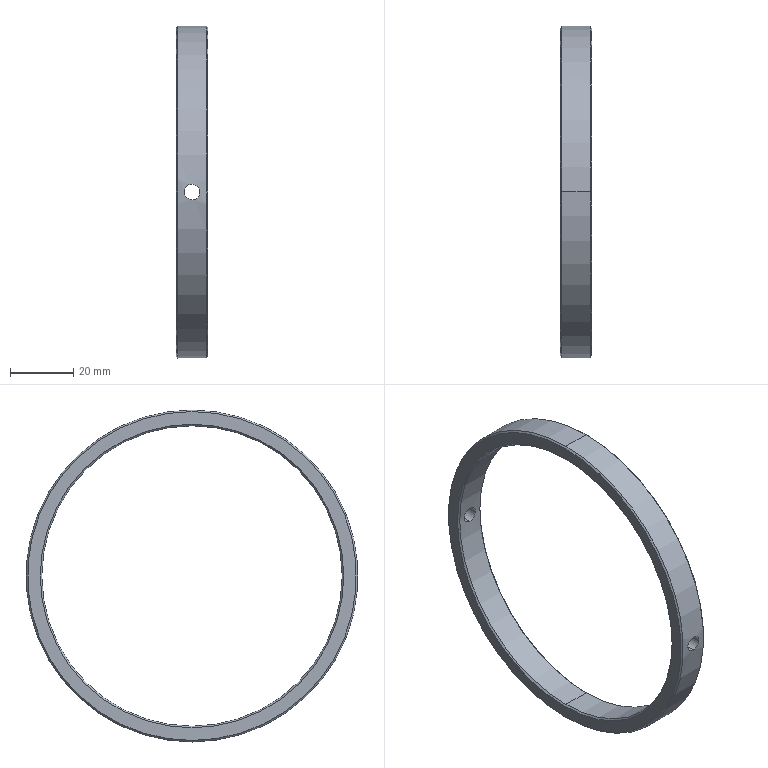Part | SolidWorks | features Chamfer 1, Extrusion 1, HoleWzd 1 | 1 solid | 18 faces | box 10 x 105 x 105 mm | volume 15354 mm3 | cylinder 8 | cone 8 | plane 2 | commonest cylinder face diameters 5 x4 95 x2 105 x2
STEP:
#1=CARTESIAN_POINT('',(0.,-52.44,-2.5));
#2=VERTEX_POINT('',#1);
#3=CARTESIAN_POINT('',(0.,-52.44,2.5));
#4=VERTEX_POINT('',#3);
#5=CARTESIAN_POINT('',(0.,-52.44,-2.5));
#6=CARTESIAN_POINT('',(-0.1649,-52.44,-2.5));
#7=CARTESIAN_POINT('',(-0.3279,-52.441,-2.484));
#8=CARTESIAN_POINT('',(-0.6473,-52.444,-2.42));
#9=CARTESIAN_POINT('',(-0.8058,-52.446,-2.372));
#10=CARTESIAN_POINT('',(-1.109,-52.452,-2.247));
#11=CARTESIAN_POINT('',(-1.252,-52.455,-2.17));
#12=CARTESIAN_POINT('',(-1.524,-52.462,-1.989));
#13=CARTESIAN_POINT('',(-1.653,-52.466,-1.883));
#14=CARTESIAN_POINT('',(-1.883,-52.474,-1.652));
#15=CARTESIAN_POINT('',(-1.987,-52.478,-1.526));
#16=CARTESIAN_POINT('',(-2.169,-52.485,-1.254));
#17=CARTESIAN_POINT('',(-2.247,-52.489,-1.108));
#18=CARTESIAN_POINT('',(-2.434,-52.497,-0.6566));
#19=CARTESIAN_POINT('',(-2.5,-52.5,-0.3283));
#20=CARTESIAN_POINT('',(-2.5,-52.5,0.1671));
#21=CARTESIAN_POINT('',(-2.484,-52.499,0.3295));
#22=CARTESIAN_POINT('',(-2.42,-52.496,0.6489));
#23=CARTESIAN_POINT('',(-2.372,-52.494,0.8076));
#24=CARTESIAN_POINT('',(-2.246,-52.488,1.11));
#25=CARTESIAN_POINT('',(-2.169,-52.485,1.254));
#26=CARTESIAN_POINT('',(-1.987,-52.478,1.525));
#27=CARTESIAN_POINT('',(-1.882,-52.474,1.654));
#28=CARTESIAN_POINT('',(-1.651,-52.466,1.884));
#29=CARTESIAN_POINT('',(-1.525,-52.462,1.988));
#30=CARTESIAN_POINT('',(-1.252,-52.455,2.17));
#31=CARTESIAN_POINT('',(-1.106,-52.452,2.248));
#32=CARTESIAN_POINT('',(-0.8055,-52.446,2.372));
#33=CARTESIAN_POINT('',(-0.6479,-52.444,2.42));
#34=CARTESIAN_POINT('',(-0.3252,-52.441,2.484));
#35=CARTESIAN_POINT('',(-0.163,-52.44,2.5));
#36=CARTESIAN_POINT('',(0.,-52.44,2.5));
#37=B_SPLINE_CURVE_WITH_KNOTS('',3,(#5,#6,#7,#8,#9,#10,#11,#12,#13,#14,#15,#16,#17,#18,#19,#20,#21,#22,#23,#24,#25,#26,#27,#28,#29,#30,#31,#32,#33,#34,#35,#36),.UNSPECIFIED.,.F.,.F.,(4,2,2,2,2,2,2,2,2,2,2,2,2,2,2,4),(0.01173,0.01222,0.0127,0.01319,0.01368,0.01417,0.01466,0.01563,0.01612,0.01661,0.0171,0.01759,0.01808,0.01857,0.01905,0.01954),.UNSPECIFIED.);
#38=EDGE_CURVE('',#2,#4,#37,.T.);
#39=ORIENTED_EDGE('',*,*,#38,.F.);
#40=CARTESIAN_POINT('',(0.,-47.434,-2.5));
#41=VERTEX_POINT('',#40);
#42=CARTESIAN_POINT('',(0.,52.5,-2.5));
#43=DIRECTION('',(0.,1.,0.));
#44=VECTOR('',#43,1000.);
#45=LINE('',#42,#44);
#46=EDGE_CURVE('',#2,#41,#45,.T.);
#47=ORIENTED_EDGE('',*,*,#46,.T.);
#48=CARTESIAN_POINT('',(0.,-47.434,2.5));
#49=VERTEX_POINT('',#48);
#50=CARTESIAN_POINT('',(0.,-47.434,-2.5));
#51=CARTESIAN_POINT('',(-0.1631,-47.434,-2.5));
#52=CARTESIAN_POINT('',(-0.3253,-47.435,-2.484));
#53=CARTESIAN_POINT('',(-0.6476,-47.438,-2.42));
#54=CARTESIAN_POINT('',(-0.8056,-47.441,-2.372));
#55=CARTESIAN_POINT('',(-1.257,-47.45,-2.185));
#56=CARTESIAN_POINT('',(-1.536,-47.458,-1.999));
#57=CARTESIAN_POINT('',(-1.882,-47.471,-1.654));
#58=CARTESIAN_POINT('',(-1.987,-47.476,-1.525));
#59=CARTESIAN_POINT('',(-2.169,-47.484,-1.254));
#60=CARTESIAN_POINT('',(-2.246,-47.487,-1.11));
#61=CARTESIAN_POINT('',(-2.372,-47.493,-0.8078));
#62=CARTESIAN_POINT('',(-2.42,-47.496,-0.6488));
#63=CARTESIAN_POINT('',(-2.484,-47.499,-0.3293));
#64=CARTESIAN_POINT('',(-2.5,-47.5,-0.167));
#65=CARTESIAN_POINT('',(-2.5,-47.5,0.1629));
#66=CARTESIAN_POINT('',(-2.484,-47.499,0.3259));
#67=CARTESIAN_POINT('',(-2.421,-47.496,0.6454));
#68=CARTESIAN_POINT('',(-2.373,-47.493,0.8039));
#69=CARTESIAN_POINT('',(-2.248,-47.487,1.107));
#70=CARTESIAN_POINT('',(-2.171,-47.484,1.251));
#71=CARTESIAN_POINT('',(-1.99,-47.476,1.522));
#72=CARTESIAN_POINT('',(-1.884,-47.471,1.651));
#73=CARTESIAN_POINT('',(-1.654,-47.463,1.882));
#74=CARTESIAN_POINT('',(-1.528,-47.459,1.985));
#75=CARTESIAN_POINT('',(-1.255,-47.451,2.168));
#76=CARTESIAN_POINT('',(-1.11,-47.447,2.246));
#77=CARTESIAN_POINT('',(-0.6585,-47.438,2.434));
#78=CARTESIAN_POINT('',(-0.3303,-47.434,2.5));
#79=CARTESIAN_POINT('',(0.,-47.434,2.5));
#80=B_SPLINE_CURVE_WITH_KNOTS('',3,(#50,#51,#52,#53,#54,#55,#56,#57,#58,#59,#60,#61,#62,#63,#64,#65,#66,#67,#68,#69,#70,#71,#72,#73,#74,#75,#76,#77,#78,#79),.UNSPECIFIED.,.F.,.F.,(4,2,2,2,2,2,2,2,2,2,2,2,2,2,4),(0.007817,0.008306,0.008794,0.009771,0.01026,0.01075,0.01124,0.01173,0.01221,0.0127,0.01319,0.01368,0.01417,0.01466,0.01563),.UNSPECIFIED.);
#81=EDGE_CURVE('',#41,#49,#80,.T.);
#82=ORIENTED_EDGE('',*,*,#81,.T.);
#83=CARTESIAN_POINT('',(0.,52.5,2.5));
#84=DIRECTION('',(0.,1.,0.));
#85=VECTOR('',#84,1000.);
#86=LINE('',#83,#85);
#87=EDGE_CURVE('',#4,#49,#86,.T.);
#88=ORIENTED_EDGE('',*,*,#87,.F.);
#89=EDGE_LOOP('',(#39,#47,#82,#88));
#90=FACE_OUTER_BOUND('',#89,.T.);
#91=CARTESIAN_POINT('',(0.,52.5,0.));
#92=DIRECTION('',(0.,1.,0.));
#93=DIRECTION('',(0.,0.,1.));
#94=AXIS2_PLACEMENT_3D('',#91,#92,#93);
#95=CYLINDRICAL_SURFACE('',#94,2.5);
#96=ADVANCED_FACE('',(#90),#95,.F.);
#97=CARTESIAN_POINT('',(0.,47.434,2.5));
#98=VERTEX_POINT('',#97);
#99=CARTESIAN_POINT('',(0.,47.434,-2.5));
#100=VERTEX_POINT('',#99);
#101=CARTESIAN_POINT('',(0.,47.434,2.5));
#102=CARTESIAN_POINT('',(-0.1652,47.434,2.5));
#103=CARTESIAN_POINT('',(-0.3277,47.435,2.484));
#104=CARTESIAN_POINT('',(-0.6472,47.438,2.42));
#105=CARTESIAN_POINT('',(-0.806,47.441,2.372));
#106=CARTESIAN_POINT('',(-1.109,47.447,2.247));
#107=CARTESIAN_POINT('',(-1.252,47.451,2.17));
#108=CARTESIAN_POINT('',(-1.524,47.458,1.988));
#109=CARTESIAN_POINT('',(-1.653,47.463,1.883));
#110=CARTESIAN_POINT('',(-1.883,47.471,1.652));
#111=CARTESIAN_POINT('',(-1.987,47.476,1.526));
#112=CARTESIAN_POINT('',(-2.17,47.484,1.253));
#113=CARTESIAN_POINT('',(-2.247,47.487,1.107));
#114=CARTESIAN_POINT('',(-2.372,47.493,0.8066));
#115=CARTESIAN_POINT('',(-2.42,47.496,0.649));
#116=CARTESIAN_POINT('',(-2.484,47.499,0.3262));
#117=CARTESIAN_POINT('',(-2.5,47.5,0.164));
#118=CARTESIAN_POINT('',(-2.5,47.5,-0.1622));
#119=CARTESIAN_POINT('',(-2.484,47.499,-0.3279));
#120=CARTESIAN_POINT('',(-2.42,47.496,-0.6485));
#121=CARTESIAN_POINT('',(-2.373,47.493,-0.8044));
#122=CARTESIAN_POINT('',(-2.247,47.487,-1.107));
#123=CARTESIAN_POINT('',(-2.169,47.484,-1.253));
#124=CARTESIAN_POINT('',(-1.988,47.476,-1.524));
#125=CARTESIAN_POINT('',(-1.885,47.471,-1.651));
#126=CARTESIAN_POINT('',(-1.651,47.463,-1.884));
#127=CARTESIAN_POINT('',(-1.525,47.458,-1.988));
#128=CARTESIAN_POINT('',(-1.254,47.451,-2.169));
#129=CARTESIAN_POINT('',(-1.108,47.447,-2.247));
#130=CARTESIAN_POINT('',(-0.8052,47.441,-2.372));
#131=CARTESIAN_POINT('',(-0.6493,47.438,-2.42));
#132=CARTESIAN_POINT('',(-0.3289,47.435,-2.484));
#133=CARTESIAN_POINT('',(-0.1632,47.434,-2.5));
#134=CARTESIAN_POINT('',(0.,47.434,-2.5));
#135=B_SPLINE_CURVE_WITH_KNOTS('',3,(#101,#102,#103,#104,#105,#106,#107,#108,#109,#110,#111,#112,#113,#114,#115,#116,#117,#118,#119,#120,#121,#122,#123,#124,#125,#126,#127,#128,#129,#130,#131,#132,#133,#134),.UNSPECIFIED.,.F.,.F.,(4,2,2,2,2,2,2,2,2,2,2,2,2,2,2,2,4),(0.,0.0004886,0.0009772,0.001466,0.001954,0.002443,0.002932,0.00342,0.003909,0.004397,0.004886,0.005375,0.005863,0.006352,0.00684,0.007329,0.007817),.UNSPECIFIED.);
#136=EDGE_CURVE('',#98,#100,#135,.T.);
#137=ORIENTED_EDGE('',*,*,#136,.T.);
#138=CARTESIAN_POINT('',(0.,52.44,-2.5));
#139=VERTEX_POINT('',#138);
#140=CARTESIAN_POINT('',(0.,52.5,-2.5));
#141=DIRECTION('',(0.,1.,0.));
#142=VECTOR('',#141,1000.);
#143=LINE('',#140,#142);
#144=EDGE_CURVE('',#100,#139,#143,.T.);
#145=ORIENTED_EDGE('',*,*,#144,.T.);
#146=CARTESIAN_POINT('',(0.,52.44,2.5));
#147=VERTEX_POINT('',#146);
#148=CARTESIAN_POINT('',(0.,52.44,2.5));
#149=CARTESIAN_POINT('',(-0.1652,52.44,2.5));
#150=CARTESIAN_POINT('',(-0.3276,52.441,2.484));
#151=CARTESIAN_POINT('',(-0.6472,52.444,2.42));
#152=CARTESIAN_POINT('',(-0.806,52.446,2.372));
#153=CARTESIAN_POINT('',(-1.109,52.452,2.247));
#154=CARTESIAN_POINT('',(-1.252,52.455,2.17));
#155=CARTESIAN_POINT('',(-1.524,52.462,1.988));
#156=CARTESIAN_POINT('',(-1.653,52.466,1.883));
#157=CARTESIAN_POINT('',(-1.883,52.474,1.652));
#158=CARTESIAN_POINT('',(-1.987,52.478,1.526));
#159=CARTESIAN_POINT('',(-2.17,52.485,1.253));
#160=CARTESIAN_POINT('',(-2.247,52.489,1.107));
#161=CARTESIAN_POINT('',(-2.372,52.494,0.8065));
#162=CARTESIAN_POINT('',(-2.42,52.496,0.649));
#163=CARTESIAN_POINT('',(-2.484,52.499,0.3262));
#164=CARTESIAN_POINT('',(-2.5,52.5,0.164));
#165=CARTESIAN_POINT('',(-2.5,52.5,-0.1622));
#166=CARTESIAN_POINT('',(-2.484,52.499,-0.3278));
#167=CARTESIAN_POINT('',(-2.42,52.496,-0.6485));
#168=CARTESIAN_POINT('',(-2.373,52.494,-0.8044));
#169=CARTESIAN_POINT('',(-2.247,52.489,-1.107));
#170=CARTESIAN_POINT('',(-2.169,52.485,-1.253));
#171=CARTESIAN_POINT('',(-1.988,52.478,-1.524));
#172=CARTESIAN_POINT('',(-1.885,52.474,-1.651));
#173=CARTESIAN_POINT('',(-1.651,52.466,-1.884));
#174=CARTESIAN_POINT('',(-1.525,52.462,-1.988));
#175=CARTESIAN_POINT('',(-1.254,52.455,-2.169));
#176=CARTESIAN_POINT('',(-1.108,52.452,-2.247));
#177=CARTESIAN_POINT('',(-0.8051,52.446,-2.372));
#178=CARTESIAN_POINT('',(-0.6493,52.444,-2.42));
#179=CARTESIAN_POINT('',(-0.3289,52.441,-2.484));
#180=CARTESIAN_POINT('',(-0.1632,52.44,-2.5));
#181=CARTESIAN_POINT('',(0.,52.44,-2.5));
#182=B_SPLINE_CURVE_WITH_KNOTS('',3,(#148,#149,#150,#151,#152,#153,#154,#155,#156,#157,#158,#159,#160,#161,#162,#163,#164,#165,#166,#167,#168,#169,#170,#171,#172,#173,#174,#175,#176,#177,#178,#179,#180,#181),.UNSPECIFIED.,.F.,.F.,(4,2,2,2,2,2,2,2,2,2,2,2,2,2,2,2,4),(0.,0.0004886,0.0009772,0.001466,0.001954,0.002443,0.002931,0.00342,0.003909,0.004397,0.004886,0.005374,0.005863,0.006352,0.00684,0.007329,0.007817),.UNSPECIFIED.);
#183=EDGE_CURVE('',#147,#139,#182,.T.);
#184=ORIENTED_EDGE('',*,*,#183,.F.);
#185=CARTESIAN_POINT('',(0.,52.5,2.5));
#186=DIRECTION('',(0.,1.,0.));
#187=VECTOR('',#186,1000.);
#188=LINE('',#185,#187);
#189=EDGE_CURVE('',#98,#147,#188,.T.);
#190=ORIENTED_EDGE('',*,*,#189,.F.);
#191=EDGE_LOOP('',(#137,#145,#184,#190));
#192=FACE_OUTER_BOUND('',#191,.T.);
#193=CARTESIAN_POINT('',(0.,52.5,0.));
#194=DIRECTION('',(0.,1.,0.));
#195=DIRECTION('',(0.,0.,1.));
#196=AXIS2_PLACEMENT_3D('',#193,#194,#195);
#197=CYLINDRICAL_SURFACE('',#196,2.5);
#198=ADVANCED_FACE('',(#192),#197,.F.);
#199=CARTESIAN_POINT('',(4.5,0.,47.5));
#200=VERTEX_POINT('',#199);
#201=CARTESIAN_POINT('',(4.5,0.,-47.5));
#202=VERTEX_POINT('',#201);
#203=CARTESIAN_POINT('',(4.5,0.,0.));
#204=DIRECTION('',(1.,0.,0.));
#205=DIRECTION('',(0.,0.,-1.));
#206=AXIS2_PLACEMENT_3D('',#203,#204,#205);
#207=CIRCLE('',#206,47.5);
#208=EDGE_CURVE('',#200,#202,#207,.T.);
#209=ORIENTED_EDGE('',*,*,#208,.F.);
#210=CARTESIAN_POINT('',(5.,0.,48.));
#211=VERTEX_POINT('',#210);
#212=CARTESIAN_POINT('',(4.5,0.,47.5));
#213=DIRECTION('',(0.7071,0.,0.7071));
#214=VECTOR('',#213,1000.);
#215=LINE('',#212,#214);
#216=EDGE_CURVE('',#200,#211,#215,.T.);
#217=ORIENTED_EDGE('',*,*,#216,.T.);
#218=CARTESIAN_POINT('',(5.,0.,-48.));
#219=VERTEX_POINT('',#218);
#220=CARTESIAN_POINT('',(5.,0.,0.));
#221=DIRECTION('',(-1.,0.,0.));
#222=DIRECTION('',(0.,0.,-1.));
#223=AXIS2_PLACEMENT_3D('',#220,#221,#222);
#224=CIRCLE('',#223,48.);
#225=EDGE_CURVE('',#219,#211,#224,.T.);
#226=ORIENTED_EDGE('',*,*,#225,.F.);
#227=CARTESIAN_POINT('',(4.5,0.,-47.5));
#228=DIRECTION('',(0.7071,0.,-0.7071));
#229=VECTOR('',#228,1000.);
#230=LINE('',#227,#229);
#231=EDGE_CURVE('',#202,#219,#230,.T.);
#232=ORIENTED_EDGE('',*,*,#231,.F.);
#233=EDGE_LOOP('',(#209,#217,#226,#232));
#234=FACE_OUTER_BOUND('',#233,.T.);
#235=CARTESIAN_POINT('',(4.5,0.,0.));
#236=DIRECTION('',(1.,0.,0.));
#237=DIRECTION('',(0.,0.,-1.));
#238=AXIS2_PLACEMENT_3D('',#235,#236,#237);
#239=CONICAL_SURFACE('',#238,47.5,0.7854);
#240=ADVANCED_FACE('',(#234),#239,.F.);
#241=CARTESIAN_POINT('',(-4.5,0.,-47.5));
#242=VERTEX_POINT('',#241);
#243=CARTESIAN_POINT('',(-4.5,0.,47.5));
#244=VERTEX_POINT('',#243);
#245=CARTESIAN_POINT('',(-4.5,0.,0.));
#246=DIRECTION('',(-1.,0.,0.));
#247=DIRECTION('',(0.,0.,-1.));
#248=AXIS2_PLACEMENT_3D('',#245,#246,#247);
#249=CIRCLE('',#248,47.5);
#250=EDGE_CURVE('',#242,#244,#249,.T.);
#251=ORIENTED_EDGE('',*,*,#250,.F.);
#252=CARTESIAN_POINT('',(-5.,0.,-48.));
#253=VERTEX_POINT('',#252);
#254=CARTESIAN_POINT('',(-5.,0.,-48.));
#255=DIRECTION('',(-0.7071,0.,-0.7071));
#256=VECTOR('',#255,1000.);
#257=LINE('',#254,#256);
#258=EDGE_CURVE('',#242,#253,#257,.T.);
#259=ORIENTED_EDGE('',*,*,#258,.T.);
#260=CARTESIAN_POINT('',(-5.,0.,48.));
#261=VERTEX_POINT('',#260);
#262=CARTESIAN_POINT('',(-5.,0.,0.));
#263=DIRECTION('',(1.,0.,0.));
#264=DIRECTION('',(0.,0.,-1.));
#265=AXIS2_PLACEMENT_3D('',#262,#263,#264);
#266=CIRCLE('',#265,48.);
#267=EDGE_CURVE('',#261,#253,#266,.T.);
#268=ORIENTED_EDGE('',*,*,#267,.F.);
#269=CARTESIAN_POINT('',(-5.,0.,48.));
#270=DIRECTION('',(-0.7071,0.,0.7071));
#271=VECTOR('',#270,1000.);
#272=LINE('',#269,#271);
#273=EDGE_CURVE('',#244,#261,#272,.T.);
#274=ORIENTED_EDGE('',*,*,#273,.F.);
#275=EDGE_LOOP('',(#251,#259,#268,#274));
#276=FACE_OUTER_BOUND('',#275,.T.);
#277=CARTESIAN_POINT('',(-5.,0.,0.));
#278=DIRECTION('',(-1.,0.,0.));
#279=DIRECTION('',(0.,0.,1.));
#280=AXIS2_PLACEMENT_3D('',#277,#278,#279);
#281=CONICAL_SURFACE('',#280,48.,0.7854);
#282=ADVANCED_FACE('',(#276),#281,.F.);
#283=CARTESIAN_POINT('',(5.,0.,-52.));
#284=VERTEX_POINT('',#283);
#285=CARTESIAN_POINT('',(5.,0.,52.));
#286=VERTEX_POINT('',#285);
#287=CARTESIAN_POINT('',(5.,0.,0.));
#288=DIRECTION('',(1.,0.,0.));
#289=DIRECTION('',(0.,0.,-1.));
#290=AXIS2_PLACEMENT_3D('',#287,#288,#289);
#291=CIRCLE('',#290,52.);
#292=EDGE_CURVE('',#284,#286,#291,.T.);
#293=ORIENTED_EDGE('',*,*,#292,.F.);
#294=CARTESIAN_POINT('',(4.5,0.,-52.5));
#295=VERTEX_POINT('',#294);
#296=CARTESIAN_POINT('',(5.,0.,-52.));
#297=DIRECTION('',(-0.7071,0.,-0.7071));
#298=VECTOR('',#297,1000.);
#299=LINE('',#296,#298);
#300=EDGE_CURVE('',#284,#295,#299,.T.);
#301=ORIENTED_EDGE('',*,*,#300,.T.);
#302=CARTESIAN_POINT('',(4.5,0.,52.5));
#303=VERTEX_POINT('',#302);
#304=CARTESIAN_POINT('',(4.5,0.,0.));
#305=DIRECTION('',(-1.,0.,0.));
#306=DIRECTION('',(0.,0.,-1.));
#307=AXIS2_PLACEMENT_3D('',#304,#305,#306);
#308=CIRCLE('',#307,52.5);
#309=EDGE_CURVE('',#303,#295,#308,.T.);
#310=ORIENTED_EDGE('',*,*,#309,.F.);
#311=CARTESIAN_POINT('',(5.,0.,52.));
#312=DIRECTION('',(-0.7071,0.,0.7071));
#313=VECTOR('',#312,1000.);
#314=LINE('',#311,#313);
#315=EDGE_CURVE('',#286,#303,#314,.T.);
#316=ORIENTED_EDGE('',*,*,#315,.F.);
#317=EDGE_LOOP('',(#293,#301,#310,#316));
#318=FACE_OUTER_BOUND('',#317,.T.);
#319=CARTESIAN_POINT('',(5.,0.,0.));
#320=DIRECTION('',(-1.,0.,0.));
#321=DIRECTION('',(0.,0.,1.));
#322=AXIS2_PLACEMENT_3D('',#319,#320,#321);
#323=CONICAL_SURFACE('',#322,52.,0.7854);
#324=ADVANCED_FACE('',(#318),#323,.T.);
#325=CARTESIAN_POINT('',(-5.,0.,52.));
#326=VERTEX_POINT('',#325);
#327=CARTESIAN_POINT('',(-5.,0.,-52.));
#328=VERTEX_POINT('',#327);
#329=CARTESIAN_POINT('',(-5.,0.,0.));
#330=DIRECTION('',(-1.,0.,0.));
#331=DIRECTION('',(0.,0.,-1.));
#332=AXIS2_PLACEMENT_3D('',#329,#330,#331);
#333=CIRCLE('',#332,52.);
#334=EDGE_CURVE('',#326,#328,#333,.T.);
#335=ORIENTED_EDGE('',*,*,#334,.F.);
#336=CARTESIAN_POINT('',(-4.5,0.,52.5));
#337=VERTEX_POINT('',#336);
#338=CARTESIAN_POINT('',(-4.5,0.,52.5));
#339=DIRECTION('',(0.7071,0.,0.7071));
#340=VECTOR('',#339,1000.);
#341=LINE('',#338,#340);
#342=EDGE_CURVE('',#326,#337,#341,.T.);
#343=ORIENTED_EDGE('',*,*,#342,.T.);
#344=CARTESIAN_POINT('',(-4.5,0.,-52.5));
#345=VERTEX_POINT('',#344);
#346=CARTESIAN_POINT('',(-4.5,0.,0.));
#347=DIRECTION('',(1.,0.,0.));
#348=DIRECTION('',(0.,0.,-1.));
#349=AXIS2_PLACEMENT_3D('',#346,#347,#348);
#350=CIRCLE('',#349,52.5);
#351=EDGE_CURVE('',#345,#337,#350,.T.);
#352=ORIENTED_EDGE('',*,*,#351,.F.);
#353=CARTESIAN_POINT('',(-4.5,0.,-52.5));
#354=DIRECTION('',(0.7071,0.,-0.7071));
#355=VECTOR('',#354,1000.);
#356=LINE('',#353,#355);
#357=EDGE_CURVE('',#328,#345,#356,.T.);
#358=ORIENTED_EDGE('',*,*,#357,.F.);
#359=EDGE_LOOP('',(#335,#343,#352,#358));
#360=FACE_OUTER_BOUND('',#359,.T.);
#361=CARTESIAN_POINT('',(-4.5,0.,0.));
#362=DIRECTION('',(1.,0.,0.));
#363=DIRECTION('',(0.,0.,-1.));
#364=AXIS2_PLACEMENT_3D('',#361,#362,#363);
#365=CONICAL_SURFACE('',#364,52.5,0.7854);
#366=ADVANCED_FACE('',(#360),#365,.T.);
#367=CARTESIAN_POINT('',(0.,-47.434,2.5));
#368=CARTESIAN_POINT('',(0.1652,-47.434,2.5));
#369=CARTESIAN_POINT('',(0.3277,-47.435,2.484));
#370=CARTESIAN_POINT('',(0.6472,-47.438,2.42));
#371=CARTESIAN_POINT('',(0.806,-47.441,2.372));
#372=CARTESIAN_POINT('',(1.109,-47.447,2.247));
#373=CARTESIAN_POINT('',(1.252,-47.451,2.17));
#374=CARTESIAN_POINT('',(1.524,-47.458,1.988));
#375=CARTESIAN_POINT('',(1.653,-47.463,1.883));
#376=CARTESIAN_POINT('',(1.883,-47.471,1.652));
#377=CARTESIAN_POINT('',(1.987,-47.476,1.526));
#378=CARTESIAN_POINT('',(2.17,-47.484,1.253));
#379=CARTESIAN_POINT('',(2.247,-47.487,1.107));
#380=CARTESIAN_POINT('',(2.372,-47.493,0.8066));
#381=CARTESIAN_POINT('',(2.42,-47.496,0.649));
#382=CARTESIAN_POINT('',(2.484,-47.499,0.3262));
#383=CARTESIAN_POINT('',(2.5,-47.5,0.164));
#384=CARTESIAN_POINT('',(2.5,-47.5,-0.1622));
#385=CARTESIAN_POINT('',(2.484,-47.499,-0.3279));
#386=CARTESIAN_POINT('',(2.42,-47.496,-0.6485));
#387=CARTESIAN_POINT('',(2.373,-47.493,-0.8044));
#388=CARTESIAN_POINT('',(2.247,-47.487,-1.107));
#389=CARTESIAN_POINT('',(2.169,-47.484,-1.253));
#390=CARTESIAN_POINT('',(1.988,-47.476,-1.524));
#391=CARTESIAN_POINT('',(1.885,-47.471,-1.651));
#392=CARTESIAN_POINT('',(1.651,-47.463,-1.884));
#393=CARTESIAN_POINT('',(1.525,-47.458,-1.988));
#394=CARTESIAN_POINT('',(1.254,-47.451,-2.169));
#395=CARTESIAN_POINT('',(1.108,-47.447,-2.247));
#396=CARTESIAN_POINT('',(0.8052,-47.441,-2.372));
#397=CARTESIAN_POINT('',(0.6493,-47.438,-2.42));
#398=CARTESIAN_POINT('',(0.3289,-47.435,-2.484));
#399=CARTESIAN_POINT('',(0.1632,-47.434,-2.5));
#400=CARTESIAN_POINT('',(0.,-47.434,-2.5));
#401=B_SPLINE_CURVE_WITH_KNOTS('',3,(#367,#368,#369,#370,#371,#372,#373,#374,#375,#376,#377,#378,#379,#380,#381,#382,#383,#384,#385,#386,#387,#388,#389,#390,#391,#392,#393,#394,#395,#396,#397,#398,#399,#400),.UNSPECIFIED.,.F.,.F.,(4,2,2,2,2,2,2,2,2,2,2,2,2,2,2,2,4),(0.,0.0004886,0.0009772,0.001466,0.001954,0.002443,0.002932,0.00342,0.003909,0.004397,0.004886,0.005375,0.005863,0.006352,0.00684,0.007329,0.007817),.UNSPECIFIED.);
#402=EDGE_CURVE('',#49,#41,#401,.T.);
#403=ORIENTED_EDGE('',*,*,#402,.F.);
#404=ORIENTED_EDGE('',*,*,#81,.F.);
#405=EDGE_LOOP('',(#403,#404));
#406=FACE_BOUND('',#405,.T.);
#407=ORIENTED_EDGE('',*,*,#208,.T.);
#408=CARTESIAN_POINT('',(5.,0.,-47.5));
#409=DIRECTION('',(-1.,0.,0.));
#410=VECTOR('',#409,1000.);
#411=LINE('',#408,#410);
#412=EDGE_CURVE('',#202,#242,#411,.T.);
#413=ORIENTED_EDGE('',*,*,#412,.T.);
#414=ORIENTED_EDGE('',*,*,#250,.T.);
#415=CARTESIAN_POINT('',(5.,0.,47.5));
#416=DIRECTION('',(-1.,0.,0.));
#417=VECTOR('',#416,1000.);
#418=LINE('',#415,#417);
#419=EDGE_CURVE('',#200,#244,#418,.T.);
#420=ORIENTED_EDGE('',*,*,#419,.F.);
#421=EDGE_LOOP('',(#407,#413,#414,#420));
#422=FACE_OUTER_BOUND('',#421,.T.);
#423=CARTESIAN_POINT('',(5.,0.,0.));
#424=DIRECTION('',(-1.,0.,0.));
#425=DIRECTION('',(0.,0.,1.));
#426=AXIS2_PLACEMENT_3D('',#423,#424,#425);
#427=CYLINDRICAL_SURFACE('',#426,47.5);
#428=ADVANCED_FACE('',(#406,#422),#427,.F.);
#429=ORIENTED_EDGE('',*,*,#183,.T.);
#430=CARTESIAN_POINT('',(0.,52.44,-2.5));
#431=CARTESIAN_POINT('',(0.1631,52.44,-2.5));
#432=CARTESIAN_POINT('',(0.3253,52.441,-2.484));
#433=CARTESIAN_POINT('',(0.6476,52.444,-2.42));
#434=CARTESIAN_POINT('',(0.8056,52.446,-2.372));
#435=CARTESIAN_POINT('',(1.257,52.455,-2.185));
#436=CARTESIAN_POINT('',(1.536,52.462,-1.999));
#437=CARTESIAN_POINT('',(1.882,52.474,-1.654));
#438=CARTESIAN_POINT('',(1.987,52.478,-1.525));
#439=CARTESIAN_POINT('',(2.169,52.485,-1.254));
#440=CARTESIAN_POINT('',(2.246,52.488,-1.11));
#441=CARTESIAN_POINT('',(2.372,52.494,-0.8078));
#442=CARTESIAN_POINT('',(2.42,52.496,-0.6488));
#443=CARTESIAN_POINT('',(2.484,52.499,-0.3293));
#444=CARTESIAN_POINT('',(2.5,52.5,-0.167));
#445=CARTESIAN_POINT('',(2.5,52.5,0.1628));
#446=CARTESIAN_POINT('',(2.484,52.499,0.3259));
#447=CARTESIAN_POINT('',(2.421,52.496,0.6454));
#448=CARTESIAN_POINT('',(2.373,52.494,0.8039));
#449=CARTESIAN_POINT('',(2.248,52.489,1.107));
#450=CARTESIAN_POINT('',(2.171,52.485,1.251));
#451=CARTESIAN_POINT('',(1.99,52.478,1.522));
#452=CARTESIAN_POINT('',(1.884,52.474,1.651));
#453=CARTESIAN_POINT('',(1.654,52.466,1.882));
#454=CARTESIAN_POINT('',(1.528,52.463,1.985));
#455=CARTESIAN_POINT('',(1.255,52.455,2.168));
#456=CARTESIAN_POINT('',(1.11,52.452,2.246));
#457=CARTESIAN_POINT('',(0.6585,52.444,2.434));
#458=CARTESIAN_POINT('',(0.3303,52.44,2.5));
#459=CARTESIAN_POINT('',(0.,52.44,2.5));
#460=B_SPLINE_CURVE_WITH_KNOTS('',3,(#430,#431,#432,#433,#434,#435,#436,#437,#438,#439,#440,#441,#442,#443,#444,#445,#446,#447,#448,#449,#450,#451,#452,#453,#454,#455,#456,#457,#458,#459),.UNSPECIFIED.,.F.,.F.,(4,2,2,2,2,2,2,2,2,2,2,2,2,2,4),(0.007817,0.008306,0.008794,0.009771,0.01026,0.01075,0.01124,0.01172,0.01221,0.0127,0.01319,0.01368,0.01417,0.01466,0.01563),.UNSPECIFIED.);
#461=EDGE_CURVE('',#139,#147,#460,.T.);
#462=ORIENTED_EDGE('',*,*,#461,.T.);
#463=EDGE_LOOP('',(#429,#462));
#464=FACE_BOUND('',#463,.T.);
#465=ORIENTED_EDGE('',*,*,#309,.T.);
#466=CARTESIAN_POINT('',(5.,0.,-52.5));
#467=DIRECTION('',(-1.,0.,0.));
#468=VECTOR('',#467,1000.);
#469=LINE('',#466,#468);
#470=EDGE_CURVE('',#295,#345,#469,.T.);
#471=ORIENTED_EDGE('',*,*,#470,.T.);
#472=ORIENTED_EDGE('',*,*,#351,.T.);
#473=CARTESIAN_POINT('',(5.,0.,52.5));
#474=DIRECTION('',(-1.,0.,0.));
#475=VECTOR('',#474,1000.);
#476=LINE('',#473,#475);
#477=EDGE_CURVE('',#303,#337,#476,.T.);
#478=ORIENTED_EDGE('',*,*,#477,.F.);
#479=EDGE_LOOP('',(#465,#471,#472,#478));
#480=FACE_OUTER_BOUND('',#479,.T.);
#481=CARTESIAN_POINT('',(5.,0.,0.));
#482=DIRECTION('',(-1.,0.,0.));
#483=DIRECTION('',(0.,0.,1.));
#484=AXIS2_PLACEMENT_3D('',#481,#482,#483);
#485=CYLINDRICAL_SURFACE('',#484,52.5);
#486=ADVANCED_FACE('',(#464,#480),#485,.T.);
#487=CARTESIAN_POINT('',(5.,0.,0.));
#488=DIRECTION('',(1.,0.,0.));
#489=DIRECTION('',(0.,0.,-1.));
#490=AXIS2_PLACEMENT_3D('',#487,#488,#489);
#491=CIRCLE('',#490,52.);
#492=EDGE_CURVE('',#286,#284,#491,.T.);
#493=ORIENTED_EDGE('',*,*,#492,.T.);
#494=ORIENTED_EDGE('',*,*,#292,.T.);
#495=EDGE_LOOP('',(#493,#494));
#496=FACE_OUTER_BOUND('',#495,.T.);
#497=ORIENTED_EDGE('',*,*,#225,.T.);
#498=CARTESIAN_POINT('',(5.,0.,0.));
#499=DIRECTION('',(-1.,0.,0.));
#500=DIRECTION('',(0.,0.,-1.));
#501=AXIS2_PLACEMENT_3D('',#498,#499,#500);
#502=CIRCLE('',#501,48.);
#503=EDGE_CURVE('',#211,#219,#502,.T.);
#504=ORIENTED_EDGE('',*,*,#503,.T.);
#505=EDGE_LOOP('',(#497,#504));
#506=FACE_BOUND('',#505,.T.);
#507=CARTESIAN_POINT('',(5.,0.,0.));
#508=DIRECTION('',(1.,0.,0.));
#509=DIRECTION('',(0.,0.,-1.));
#510=AXIS2_PLACEMENT_3D('',#507,#508,#509);
#511=PLANE('',#510);
#512=ADVANCED_FACE('',(#496,#506),#511,.T.);
#513=CARTESIAN_POINT('',(-5.,0.,0.));
#514=DIRECTION('',(-1.,0.,0.));
#515=DIRECTION('',(0.,0.,-1.));
#516=AXIS2_PLACEMENT_3D('',#513,#514,#515);
#517=CIRCLE('',#516,52.);
#518=EDGE_CURVE('',#328,#326,#517,.T.);
#519=ORIENTED_EDGE('',*,*,#518,.T.);
#520=ORIENTED_EDGE('',*,*,#334,.T.);
#521=EDGE_LOOP('',(#519,#520));
#522=FACE_OUTER_BOUND('',#521,.T.);
#523=ORIENTED_EDGE('',*,*,#267,.T.);
#524=CARTESIAN_POINT('',(-5.,0.,0.));
#525=DIRECTION('',(1.,0.,0.));
#526=DIRECTION('',(0.,0.,-1.));
#527=AXIS2_PLACEMENT_3D('',#524,#525,#526);
#528=CIRCLE('',#527,48.);
#529=EDGE_CURVE('',#253,#261,#528,.T.);
#530=ORIENTED_EDGE('',*,*,#529,.T.);
#531=EDGE_LOOP('',(#523,#530));
#532=FACE_BOUND('',#531,.T.);
#533=CARTESIAN_POINT('',(-5.,0.,0.));
#534=DIRECTION('',(1.,0.,0.));
#535=DIRECTION('',(0.,0.,-1.));
#536=AXIS2_PLACEMENT_3D('',#533,#534,#535);
#537=PLANE('',#536);
#538=ADVANCED_FACE('',(#522,#532),#537,.F.);
#539=ORIENTED_EDGE('',*,*,#470,.F.);
#540=CARTESIAN_POINT('',(4.5,0.,0.));
#541=DIRECTION('',(-1.,0.,0.));
#542=DIRECTION('',(0.,0.,-1.));
#543=AXIS2_PLACEMENT_3D('',#540,#541,#542);
#544=CIRCLE('',#543,52.5);
#545=EDGE_CURVE('',#295,#303,#544,.T.);
#546=ORIENTED_EDGE('',*,*,#545,.T.);
#547=ORIENTED_EDGE('',*,*,#477,.T.);
#548=CARTESIAN_POINT('',(-4.5,0.,0.));
#549=DIRECTION('',(1.,0.,0.));
#550=DIRECTION('',(0.,0.,-1.));
#551=AXIS2_PLACEMENT_3D('',#548,#549,#550);
#552=CIRCLE('',#551,52.5);
#553=EDGE_CURVE('',#337,#345,#552,.T.);
#554=ORIENTED_EDGE('',*,*,#553,.T.);
#555=EDGE_LOOP('',(#539,#546,#547,#554));
#556=FACE_OUTER_BOUND('',#555,.T.);
#557=CARTESIAN_POINT('',(0.,-52.44,2.5));
#558=CARTESIAN_POINT('',(0.1631,-52.44,2.5));
#559=CARTESIAN_POINT('',(0.3287,-52.441,2.484));
#560=CARTESIAN_POINT('',(0.6494,-52.444,2.42));
#561=CARTESIAN_POINT('',(0.8052,-52.446,2.372));
#562=CARTESIAN_POINT('',(1.108,-52.452,2.247));
#563=CARTESIAN_POINT('',(1.254,-52.455,2.169));
#564=CARTESIAN_POINT('',(1.525,-52.462,1.988));
#565=CARTESIAN_POINT('',(1.651,-52.466,1.884));
#566=CARTESIAN_POINT('',(1.885,-52.474,1.651));
#567=CARTESIAN_POINT('',(1.988,-52.478,1.524));
#568=CARTESIAN_POINT('',(2.169,-52.485,1.253));
#569=CARTESIAN_POINT('',(2.247,-52.489,1.107));
#570=CARTESIAN_POINT('',(2.373,-52.494,0.8042));
#571=CARTESIAN_POINT('',(2.42,-52.496,0.6483));
#572=CARTESIAN_POINT('',(2.484,-52.499,0.3279));
#573=CARTESIAN_POINT('',(2.5,-52.5,0.1622));
#574=CARTESIAN_POINT('',(2.5,-52.5,-0.1642));
#575=CARTESIAN_POINT('',(2.484,-52.499,-0.3264));
#576=CARTESIAN_POINT('',(2.42,-52.496,-0.6487));
#577=CARTESIAN_POINT('',(2.372,-52.494,-0.8067));
#578=CARTESIAN_POINT('',(2.185,-52.486,-1.258));
#579=CARTESIAN_POINT('',(1.998,-52.478,-1.537));
#580=CARTESIAN_POINT('',(1.653,-52.466,-1.883));
#581=CARTESIAN_POINT('',(1.524,-52.462,-1.988));
#582=CARTESIAN_POINT('',(1.252,-52.455,-2.17));
#583=CARTESIAN_POINT('',(1.109,-52.452,-2.247));
#584=CARTESIAN_POINT('',(0.806,-52.446,-2.372));
#585=CARTESIAN_POINT('',(0.647,-52.444,-2.42));
#586=CARTESIAN_POINT('',(0.3273,-52.441,-2.484));
#587=CARTESIAN_POINT('',(0.165,-52.44,-2.5));
#588=CARTESIAN_POINT('',(0.,-52.44,-2.5));
#589=B_SPLINE_CURVE_WITH_KNOTS('',3,(#557,#558,#559,#560,#561,#562,#563,#564,#565,#566,#567,#568,#569,#570,#571,#572,#573,#574,#575,#576,#577,#578,#579,#580,#581,#582,#583,#584,#585,#586,#587,#588),.UNSPECIFIED.,.F.,.F.,(4,2,2,2,2,2,2,2,2,2,2,2,2,2,2,4),(0.00391,0.004398,0.004887,0.005375,0.005864,0.006352,0.006841,0.00733,0.007818,0.008307,0.008795,0.009773,0.01026,0.01075,0.01124,0.01173),.UNSPECIFIED.);
#590=EDGE_CURVE('',#4,#2,#589,.T.);
#591=ORIENTED_EDGE('',*,*,#590,.T.);
#592=ORIENTED_EDGE('',*,*,#38,.T.);
#593=EDGE_LOOP('',(#591,#592));
#594=FACE_BOUND('',#593,.T.);
#595=CARTESIAN_POINT('',(5.,0.,0.));
#596=DIRECTION('',(-1.,0.,0.));
#597=DIRECTION('',(0.,0.,1.));
#598=AXIS2_PLACEMENT_3D('',#595,#596,#597);
#599=CYLINDRICAL_SURFACE('',#598,52.5);
#600=ADVANCED_FACE('',(#556,#594),#599,.T.);
#601=ORIENTED_EDGE('',*,*,#412,.F.);
#602=CARTESIAN_POINT('',(4.5,0.,0.));
#603=DIRECTION('',(1.,0.,0.));
#604=DIRECTION('',(0.,0.,-1.));
#605=AXIS2_PLACEMENT_3D('',#602,#603,#604);
#606=CIRCLE('',#605,47.5);
#607=EDGE_CURVE('',#202,#200,#606,.T.);
#608=ORIENTED_EDGE('',*,*,#607,.T.);
#609=ORIENTED_EDGE('',*,*,#419,.T.);
#610=CARTESIAN_POINT('',(-4.5,0.,0.));
#611=DIRECTION('',(-1.,0.,0.));
#612=DIRECTION('',(0.,0.,-1.));
#613=AXIS2_PLACEMENT_3D('',#610,#611,#612);
#614=CIRCLE('',#613,47.5);
#615=EDGE_CURVE('',#244,#242,#614,.T.);
#616=ORIENTED_EDGE('',*,*,#615,.T.);
#617=EDGE_LOOP('',(#601,#608,#609,#616));
#618=FACE_OUTER_BOUND('',#617,.T.);
#619=ORIENTED_EDGE('',*,*,#136,.F.);
#620=CARTESIAN_POINT('',(0.,47.434,-2.5));
#621=CARTESIAN_POINT('',(0.1631,47.434,-2.5));
#622=CARTESIAN_POINT('',(0.3253,47.435,-2.484));
#623=CARTESIAN_POINT('',(0.6476,47.438,-2.42));
#624=CARTESIAN_POINT('',(0.8056,47.441,-2.372));
#625=CARTESIAN_POINT('',(1.257,47.45,-2.185));
#626=CARTESIAN_POINT('',(1.536,47.458,-1.999));
#627=CARTESIAN_POINT('',(1.882,47.471,-1.654));
#628=CARTESIAN_POINT('',(1.987,47.476,-1.525));
#629=CARTESIAN_POINT('',(2.169,47.484,-1.254));
#630=CARTESIAN_POINT('',(2.246,47.487,-1.11));
#631=CARTESIAN_POINT('',(2.372,47.493,-0.8078));
#632=CARTESIAN_POINT('',(2.42,47.496,-0.6488));
#633=CARTESIAN_POINT('',(2.484,47.499,-0.3293));
#634=CARTESIAN_POINT('',(2.5,47.5,-0.167));
#635=CARTESIAN_POINT('',(2.5,47.5,0.1629));
#636=CARTESIAN_POINT('',(2.484,47.499,0.3259));
#637=CARTESIAN_POINT('',(2.421,47.496,0.6454));
#638=CARTESIAN_POINT('',(2.373,47.493,0.8039));
#639=CARTESIAN_POINT('',(2.248,47.487,1.107));
#640=CARTESIAN_POINT('',(2.171,47.484,1.251));
#641=CARTESIAN_POINT('',(1.99,47.476,1.522));
#642=CARTESIAN_POINT('',(1.884,47.471,1.651));
#643=CARTESIAN_POINT('',(1.654,47.463,1.882));
#644=CARTESIAN_POINT('',(1.528,47.459,1.985));
#645=CARTESIAN_POINT('',(1.255,47.451,2.168));
#646=CARTESIAN_POINT('',(1.11,47.447,2.246));
#647=CARTESIAN_POINT('',(0.6585,47.438,2.434));
#648=CARTESIAN_POINT('',(0.3303,47.434,2.5));
#649=CARTESIAN_POINT('',(0.,47.434,2.5));
#650=B_SPLINE_CURVE_WITH_KNOTS('',3,(#620,#621,#622,#623,#624,#625,#626,#627,#628,#629,#630,#631,#632,#633,#634,#635,#636,#637,#638,#639,#640,#641,#642,#643,#644,#645,#646,#647,#648,#649),.UNSPECIFIED.,.F.,.F.,(4,2,2,2,2,2,2,2,2,2,2,2,2,2,4),(0.007817,0.008306,0.008794,0.009771,0.01026,0.01075,0.01124,0.01173,0.01221,0.0127,0.01319,0.01368,0.01417,0.01466,0.01563),.UNSPECIFIED.);
#651=EDGE_CURVE('',#100,#98,#650,.T.);
#652=ORIENTED_EDGE('',*,*,#651,.F.);
#653=EDGE_LOOP('',(#619,#652));
#654=FACE_BOUND('',#653,.T.);
#655=CARTESIAN_POINT('',(5.,0.,0.));
#656=DIRECTION('',(-1.,0.,0.));
#657=DIRECTION('',(0.,0.,1.));
#658=AXIS2_PLACEMENT_3D('',#655,#656,#657);
#659=CYLINDRICAL_SURFACE('',#658,47.5);
#660=ADVANCED_FACE('',(#618,#654),#659,.F.);
#661=ORIENTED_EDGE('',*,*,#342,.F.);
#662=ORIENTED_EDGE('',*,*,#518,.F.);
#663=ORIENTED_EDGE('',*,*,#357,.T.);
#664=ORIENTED_EDGE('',*,*,#553,.F.);
#665=EDGE_LOOP('',(#661,#662,#663,#664));
#666=FACE_OUTER_BOUND('',#665,.T.);
#667=CARTESIAN_POINT('',(-4.5,0.,0.));
#668=DIRECTION('',(1.,0.,0.));
#669=DIRECTION('',(0.,0.,-1.));
#670=AXIS2_PLACEMENT_3D('',#667,#668,#669);
#671=CONICAL_SURFACE('',#670,52.5,0.7854);
#672=ADVANCED_FACE('',(#666),#671,.T.);
#673=ORIENTED_EDGE('',*,*,#300,.F.);
#674=ORIENTED_EDGE('',*,*,#492,.F.);
#675=ORIENTED_EDGE('',*,*,#315,.T.);
#676=ORIENTED_EDGE('',*,*,#545,.F.);
#677=EDGE_LOOP('',(#673,#674,#675,#676));
#678=FACE_OUTER_BOUND('',#677,.T.);
#679=CARTESIAN_POINT('',(5.,0.,0.));
#680=DIRECTION('',(-1.,0.,0.));
#681=DIRECTION('',(0.,0.,1.));
#682=AXIS2_PLACEMENT_3D('',#679,#680,#681);
#683=CONICAL_SURFACE('',#682,52.,0.7854);
#684=ADVANCED_FACE('',(#678),#683,.T.);
#685=ORIENTED_EDGE('',*,*,#258,.F.);
#686=ORIENTED_EDGE('',*,*,#615,.F.);
#687=ORIENTED_EDGE('',*,*,#273,.T.);
#688=ORIENTED_EDGE('',*,*,#529,.F.);
#689=EDGE_LOOP('',(#685,#686,#687,#688));
#690=FACE_OUTER_BOUND('',#689,.T.);
#691=CARTESIAN_POINT('',(-5.,0.,0.));
#692=DIRECTION('',(-1.,0.,0.));
#693=DIRECTION('',(0.,0.,1.));
#694=AXIS2_PLACEMENT_3D('',#691,#692,#693);
#695=CONICAL_SURFACE('',#694,48.,0.7854);
#696=ADVANCED_FACE('',(#690),#695,.F.);
#697=ORIENTED_EDGE('',*,*,#216,.F.);
#698=ORIENTED_EDGE('',*,*,#607,.F.);
#699=ORIENTED_EDGE('',*,*,#231,.T.);
#700=ORIENTED_EDGE('',*,*,#503,.F.);
#701=EDGE_LOOP('',(#697,#698,#699,#700));
#702=FACE_OUTER_BOUND('',#701,.T.);
#703=CARTESIAN_POINT('',(4.5,0.,0.));
#704=DIRECTION('',(1.,0.,0.));
#705=DIRECTION('',(0.,0.,-1.));
#706=AXIS2_PLACEMENT_3D('',#703,#704,#705);
#707=CONICAL_SURFACE('',#706,47.5,0.7854);
#708=ADVANCED_FACE('',(#702),#707,.F.);
#709=ORIENTED_EDGE('',*,*,#144,.F.);
#710=ORIENTED_EDGE('',*,*,#651,.T.);
#711=ORIENTED_EDGE('',*,*,#189,.T.);
#712=ORIENTED_EDGE('',*,*,#461,.F.);
#713=EDGE_LOOP('',(#709,#710,#711,#712));
#714=FACE_OUTER_BOUND('',#713,.T.);
#715=CARTESIAN_POINT('',(0.,52.5,0.));
#716=DIRECTION('',(0.,1.,0.));
#717=DIRECTION('',(0.,0.,1.));
#718=AXIS2_PLACEMENT_3D('',#715,#716,#717);
#719=CYLINDRICAL_SURFACE('',#718,2.5);
#720=ADVANCED_FACE('',(#714),#719,.F.);
#721=ORIENTED_EDGE('',*,*,#46,.F.);
#722=ORIENTED_EDGE('',*,*,#590,.F.);
#723=ORIENTED_EDGE('',*,*,#87,.T.);
#724=ORIENTED_EDGE('',*,*,#402,.T.);
#725=EDGE_LOOP('',(#721,#722,#723,#724));
#726=FACE_OUTER_BOUND('',#725,.T.);
#727=CARTESIAN_POINT('',(0.,52.5,0.));
#728=DIRECTION('',(0.,1.,0.));
#729=DIRECTION('',(0.,0.,1.));
#730=AXIS2_PLACEMENT_3D('',#727,#728,#729);
#731=CYLINDRICAL_SURFACE('',#730,2.5);
#732=ADVANCED_FACE('',(#726),#731,.F.);
#733=CLOSED_SHELL('',(#96,#198,#240,#282,#324,#366,#428,#486,#512,#538,#600,#660,#672,#684,#696,#708,#720,#732));
#734=MANIFOLD_SOLID_BREP('',#733);
#735=CARTESIAN_POINT('',(0.,0.,0.));
#736=DIRECTION('',(0.,0.,1.));
#737=DIRECTION('',(1.,0.,0.));
#738=AXIS2_PLACEMENT_3D('',#735,#736,#737);
#739=(LENGTH_UNIT()NAMED_UNIT(*)SI_UNIT(.MILLI.,.METRE.));
#740=UNCERTAINTY_MEASURE_WITH_UNIT(LENGTH_MEASURE(0.00001),#739,'','');
#741=(NAMED_UNIT(*)PLANE_ANGLE_UNIT()SI_UNIT($,.RADIAN.));
#742=(NAMED_UNIT(*)SI_UNIT($,.STERADIAN.)SOLID_ANGLE_UNIT());
#743=(GEOMETRIC_REPRESENTATION_CONTEXT(3)GLOBAL_UNCERTAINTY_ASSIGNED_CONTEXT((#740))GLOBAL_UNIT_ASSIGNED_CONTEXT((#739,#741,#742))REPRESENTATION_CONTEXT('',''));
#744=ADVANCED_BREP_SHAPE_REPRESENTATION('',(#734,#738),#743);